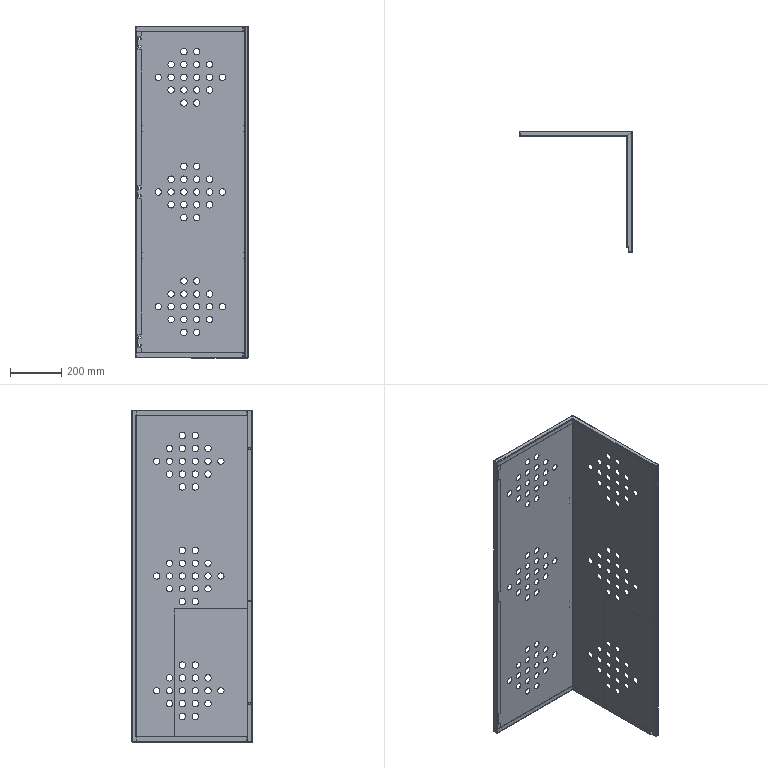Part | NX | features solid 2 | 1 solid | 426 faces | box 437 x 473 x 1295 mm | volume 1893390 mm3 | cylinder 280 | plane 138 | spline 8 | commonest cylinder face diameters 25 x216 1 x16 6 x15 3 x13 7 x12 7.2 x6